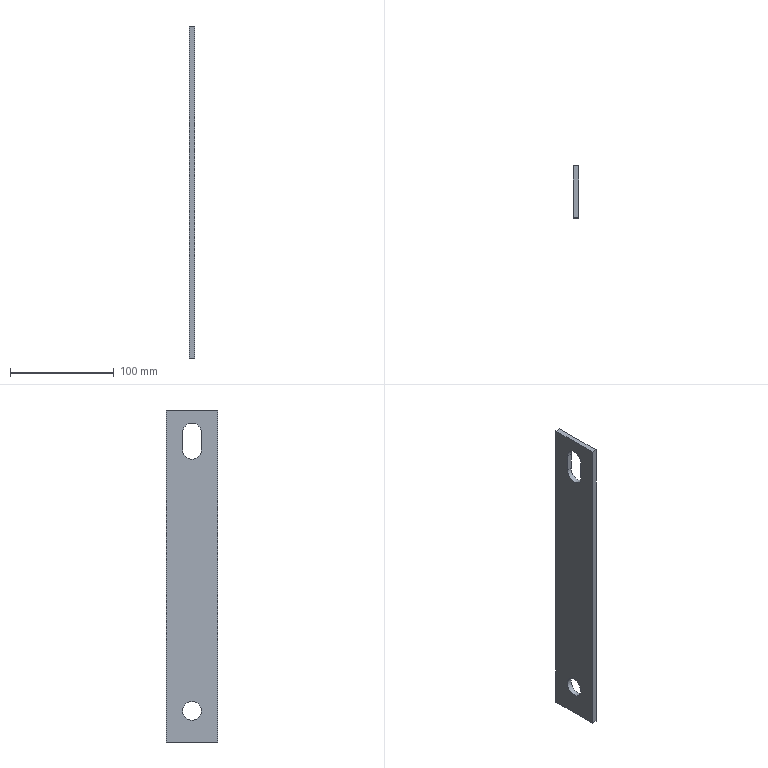Part | NX | features solid 2 | 1 solid | 11 faces | box 5 x 50 x 320 mm | volume 75925 mm3 | plane 8 | cylinder 3 | commonest cylinder face diameters 18 x3
STEP:
#1=CARTESIAN_POINT('',(-1310.,-435.,-90.));
#2=VERTEX_POINT('',#1);
#3=CARTESIAN_POINT('',(-1310.,-485.,-90.));
#4=VERTEX_POINT('',#3);
#5=CARTESIAN_POINT('',(-1310.,-460.,-90.));
#6=DIRECTION('',(0.,-1.,0.));
#7=VECTOR('',#6,1000.);
#8=LINE('',#5,#7);
#9=EDGE_CURVE('',#2,#4,#8,.T.);
#10=ORIENTED_EDGE('',*,*,#9,.T.);
#11=CARTESIAN_POINT('',(-1315.,-485.,-90.));
#12=VERTEX_POINT('',#11);
#13=CARTESIAN_POINT('',(-1312.5,-485.,-90.));
#14=DIRECTION('',(-1.,0.,0.));
#15=VECTOR('',#14,1000.);
#16=LINE('',#13,#15);
#17=EDGE_CURVE('',#4,#12,#16,.T.);
#18=ORIENTED_EDGE('',*,*,#17,.T.);
#19=CARTESIAN_POINT('',(-1315.,-435.,-90.));
#20=VERTEX_POINT('',#19);
#21=CARTESIAN_POINT('',(-1315.,-460.,-90.));
#22=DIRECTION('',(0.,1.,0.));
#23=VECTOR('',#22,1000.);
#24=LINE('',#21,#23);
#25=EDGE_CURVE('',#12,#20,#24,.T.);
#26=ORIENTED_EDGE('',*,*,#25,.T.);
#27=CARTESIAN_POINT('',(-1312.5,-435.,-90.));
#28=DIRECTION('',(1.,0.,0.));
#29=VECTOR('',#28,1000.);
#30=LINE('',#27,#29);
#31=EDGE_CURVE('',#20,#2,#30,.T.);
#32=ORIENTED_EDGE('',*,*,#31,.T.);
#33=EDGE_LOOP('',(#10,#18,#26,#32));
#34=FACE_BOUND('',#33,.T.);
#35=CARTESIAN_POINT('',(-1312.5,-460.,-90.));
#36=DIRECTION('',(0.,0.,-1.));
#37=DIRECTION('',(-1.,0.,0.));
#38=AXIS2_PLACEMENT_3D('',#35,#36,#37);
#39=PLANE('',#38);
#40=ADVANCED_FACE('',(#34),#39,.T.);
#41=CARTESIAN_POINT('',(-1315.,-460.,-69.));
#42=VERTEX_POINT('',#41);
#43=CARTESIAN_POINT('',(-1315.,-460.,-60.));
#44=DIRECTION('',(-1.,0.,0.));
#45=DIRECTION('',(0.,0.,-1.));
#46=AXIS2_PLACEMENT_3D('',#43,#44,#45);
#47=CIRCLE('',#46,9.);
#48=EDGE_CURVE('',#42,#42,#47,.T.);
#49=ORIENTED_EDGE('',*,*,#48,.T.);
#50=EDGE_LOOP('',(#49));
#51=FACE_BOUND('',#50,.T.);
#52=CARTESIAN_POINT('',(-1310.,-460.,-51.));
#53=VERTEX_POINT('',#52);
#54=CARTESIAN_POINT('',(-1310.,-460.,-60.));
#55=DIRECTION('',(1.,0.,0.));
#56=DIRECTION('',(0.,0.,1.));
#57=AXIS2_PLACEMENT_3D('',#54,#55,#56);
#58=CIRCLE('',#57,9.);
#59=EDGE_CURVE('',#53,#53,#58,.T.);
#60=ORIENTED_EDGE('',*,*,#59,.T.);
#61=EDGE_LOOP('',(#60));
#62=FACE_BOUND('',#61,.T.);
#63=CARTESIAN_POINT('',(-1310.,-460.,-60.));
#64=DIRECTION('',(-1.,0.,0.));
#65=DIRECTION('',(0.,0.,1.));
#66=AXIS2_PLACEMENT_3D('',#63,#64,#65);
#67=CYLINDRICAL_SURFACE('',#66,9.);
#68=ADVANCED_FACE('',(#51,#62),#67,.F.);
#69=ORIENTED_EDGE('',*,*,#59,.F.);
#70=EDGE_LOOP('',(#69));
#71=FACE_BOUND('',#70,.T.);
#72=CARTESIAN_POINT('',(-1310.,-485.,230.));
#73=VERTEX_POINT('',#72);
#74=CARTESIAN_POINT('',(-1310.,-485.,-120.));
#75=DIRECTION('',(0.,0.,1.));
#76=VECTOR('',#75,1000.);
#77=LINE('',#74,#76);
#78=EDGE_CURVE('',#4,#73,#77,.T.);
#79=ORIENTED_EDGE('',*,*,#78,.F.);
#80=ORIENTED_EDGE('',*,*,#9,.F.);
#81=CARTESIAN_POINT('',(-1310.,-435.,230.));
#82=VERTEX_POINT('',#81);
#83=CARTESIAN_POINT('',(-1310.,-435.,-120.));
#84=DIRECTION('',(0.,0.,1.));
#85=VECTOR('',#84,1000.);
#86=LINE('',#83,#85);
#87=EDGE_CURVE('',#2,#82,#86,.T.);
#88=ORIENTED_EDGE('',*,*,#87,.T.);
#89=CARTESIAN_POINT('',(-1310.,-460.,230.));
#90=DIRECTION('',(0.,1.,0.));
#91=VECTOR('',#90,1000.);
#92=LINE('',#89,#91);
#93=EDGE_CURVE('',#73,#82,#92,.T.);
#94=ORIENTED_EDGE('',*,*,#93,.F.);
#95=EDGE_LOOP('',(#79,#80,#88,#94));
#96=FACE_BOUND('',#95,.T.);
#97=CARTESIAN_POINT('',(-1310.,-451.,191.5));
#98=VERTEX_POINT('',#97);
#99=CARTESIAN_POINT('',(-1310.,-451.,208.5));
#100=VERTEX_POINT('',#99);
#101=CARTESIAN_POINT('',(-1310.,-451.,191.5));
#102=DIRECTION('',(0.,0.,1.));
#103=VECTOR('',#102,1000.);
#104=LINE('',#101,#103);
#105=EDGE_CURVE('',#98,#100,#104,.T.);
#106=ORIENTED_EDGE('',*,*,#105,.F.);
#107=CARTESIAN_POINT('',(-1310.,-469.,191.5));
#108=VERTEX_POINT('',#107);
#109=CARTESIAN_POINT('',(-1310.,-460.,191.5));
#110=DIRECTION('',(1.,0.,0.));
#111=DIRECTION('',(0.,0.,1.));
#112=AXIS2_PLACEMENT_3D('',#109,#110,#111);
#113=CIRCLE('',#112,9.);
#114=EDGE_CURVE('',#108,#98,#113,.T.);
#115=ORIENTED_EDGE('',*,*,#114,.F.);
#116=CARTESIAN_POINT('',(-1310.,-469.,208.5));
#117=VERTEX_POINT('',#116);
#118=CARTESIAN_POINT('',(-1310.,-469.,191.5));
#119=DIRECTION('',(0.,0.,1.));
#120=VECTOR('',#119,1000.);
#121=LINE('',#118,#120);
#122=EDGE_CURVE('',#108,#117,#121,.T.);
#123=ORIENTED_EDGE('',*,*,#122,.T.);
#124=CARTESIAN_POINT('',(-1310.,-460.,208.5));
#125=DIRECTION('',(1.,0.,0.));
#126=DIRECTION('',(0.,0.,1.));
#127=AXIS2_PLACEMENT_3D('',#124,#125,#126);
#128=CIRCLE('',#127,9.);
#129=EDGE_CURVE('',#100,#117,#128,.T.);
#130=ORIENTED_EDGE('',*,*,#129,.F.);
#131=EDGE_LOOP('',(#106,#115,#123,#130));
#132=FACE_BOUND('',#131,.T.);
#133=CARTESIAN_POINT('',(-1310.,-460.,-120.));
#134=DIRECTION('',(1.,0.,0.));
#135=DIRECTION('',(0.,0.,-1.));
#136=AXIS2_PLACEMENT_3D('',#133,#134,#135);
#137=PLANE('',#136);
#138=ADVANCED_FACE('',(#71,#96,#132),#137,.T.);
#139=CARTESIAN_POINT('',(-1315.,-485.,230.));
#140=VERTEX_POINT('',#139);
#141=CARTESIAN_POINT('',(-1315.,-485.,-120.));
#142=DIRECTION('',(0.,0.,1.));
#143=VECTOR('',#142,1000.);
#144=LINE('',#141,#143);
#145=EDGE_CURVE('',#12,#140,#144,.T.);
#146=ORIENTED_EDGE('',*,*,#145,.F.);
#147=ORIENTED_EDGE('',*,*,#17,.F.);
#148=ORIENTED_EDGE('',*,*,#78,.T.);
#149=CARTESIAN_POINT('',(-1312.5,-485.,230.));
#150=DIRECTION('',(1.,0.,0.));
#151=VECTOR('',#150,1000.);
#152=LINE('',#149,#151);
#153=EDGE_CURVE('',#140,#73,#152,.T.);
#154=ORIENTED_EDGE('',*,*,#153,.F.);
#155=EDGE_LOOP('',(#146,#147,#148,#154));
#156=FACE_BOUND('',#155,.T.);
#157=CARTESIAN_POINT('',(-1312.5,-485.,-120.));
#158=DIRECTION('',(0.,-1.,0.));
#159=DIRECTION('',(0.,0.,1.));
#160=AXIS2_PLACEMENT_3D('',#157,#158,#159);
#161=PLANE('',#160);
#162=ADVANCED_FACE('',(#156),#161,.T.);
#163=ORIENTED_EDGE('',*,*,#48,.F.);
#164=EDGE_LOOP('',(#163));
#165=FACE_BOUND('',#164,.T.);
#166=CARTESIAN_POINT('',(-1315.,-435.,230.));
#167=VERTEX_POINT('',#166);
#168=CARTESIAN_POINT('',(-1315.,-435.,-120.));
#169=DIRECTION('',(0.,0.,1.));
#170=VECTOR('',#169,1000.);
#171=LINE('',#168,#170);
#172=EDGE_CURVE('',#20,#167,#171,.T.);
#173=ORIENTED_EDGE('',*,*,#172,.F.);
#174=ORIENTED_EDGE('',*,*,#25,.F.);
#175=ORIENTED_EDGE('',*,*,#145,.T.);
#176=CARTESIAN_POINT('',(-1315.,-460.,230.));
#177=DIRECTION('',(0.,-1.,0.));
#178=VECTOR('',#177,1000.);
#179=LINE('',#176,#178);
#180=EDGE_CURVE('',#167,#140,#179,.T.);
#181=ORIENTED_EDGE('',*,*,#180,.F.);
#182=EDGE_LOOP('',(#173,#174,#175,#181));
#183=FACE_BOUND('',#182,.T.);
#184=CARTESIAN_POINT('',(-1315.,-451.,191.5));
#185=VERTEX_POINT('',#184);
#186=CARTESIAN_POINT('',(-1315.,-451.,208.5));
#187=VERTEX_POINT('',#186);
#188=CARTESIAN_POINT('',(-1315.,-451.,191.5));
#189=DIRECTION('',(0.,0.,1.));
#190=VECTOR('',#189,1000.);
#191=LINE('',#188,#190);
#192=EDGE_CURVE('',#185,#187,#191,.T.);
#193=ORIENTED_EDGE('',*,*,#192,.T.);
#194=CARTESIAN_POINT('',(-1315.,-469.,208.5));
#195=VERTEX_POINT('',#194);
#196=CARTESIAN_POINT('',(-1315.,-460.,208.5));
#197=DIRECTION('',(-1.,0.,0.));
#198=DIRECTION('',(0.,0.,-1.));
#199=AXIS2_PLACEMENT_3D('',#196,#197,#198);
#200=CIRCLE('',#199,9.);
#201=EDGE_CURVE('',#195,#187,#200,.T.);
#202=ORIENTED_EDGE('',*,*,#201,.F.);
#203=CARTESIAN_POINT('',(-1315.,-469.,191.5));
#204=VERTEX_POINT('',#203);
#205=CARTESIAN_POINT('',(-1315.,-469.,191.5));
#206=DIRECTION('',(0.,0.,1.));
#207=VECTOR('',#206,1000.);
#208=LINE('',#205,#207);
#209=EDGE_CURVE('',#204,#195,#208,.T.);
#210=ORIENTED_EDGE('',*,*,#209,.F.);
#211=CARTESIAN_POINT('',(-1315.,-460.,191.5));
#212=DIRECTION('',(-1.,0.,0.));
#213=DIRECTION('',(0.,0.,-1.));
#214=AXIS2_PLACEMENT_3D('',#211,#212,#213);
#215=CIRCLE('',#214,9.);
#216=EDGE_CURVE('',#185,#204,#215,.T.);
#217=ORIENTED_EDGE('',*,*,#216,.F.);
#218=EDGE_LOOP('',(#193,#202,#210,#217));
#219=FACE_BOUND('',#218,.T.);
#220=CARTESIAN_POINT('',(-1315.,-460.,-120.));
#221=DIRECTION('',(-1.,0.,0.));
#222=DIRECTION('',(0.,0.,1.));
#223=AXIS2_PLACEMENT_3D('',#220,#221,#222);
#224=PLANE('',#223);
#225=ADVANCED_FACE('',(#165,#183,#219),#224,.T.);
#226=ORIENTED_EDGE('',*,*,#87,.F.);
#227=ORIENTED_EDGE('',*,*,#31,.F.);
#228=ORIENTED_EDGE('',*,*,#172,.T.);
#229=CARTESIAN_POINT('',(-1312.5,-435.,230.));
#230=DIRECTION('',(-1.,0.,0.));
#231=VECTOR('',#230,1000.);
#232=LINE('',#229,#231);
#233=EDGE_CURVE('',#82,#167,#232,.T.);
#234=ORIENTED_EDGE('',*,*,#233,.F.);
#235=EDGE_LOOP('',(#226,#227,#228,#234));
#236=FACE_BOUND('',#235,.T.);
#237=CARTESIAN_POINT('',(-1312.5,-435.,-120.));
#238=DIRECTION('',(0.,1.,0.));
#239=DIRECTION('',(0.,0.,-1.));
#240=AXIS2_PLACEMENT_3D('',#237,#238,#239);
#241=PLANE('',#240);
#242=ADVANCED_FACE('',(#236),#241,.T.);
#243=CARTESIAN_POINT('',(-1312.5,-451.,208.5));
#244=DIRECTION('',(-1.,0.,0.));
#245=VECTOR('',#244,1000.);
#246=LINE('',#243,#245);
#247=EDGE_CURVE('',#100,#187,#246,.T.);
#248=ORIENTED_EDGE('',*,*,#247,.F.);
#249=ORIENTED_EDGE('',*,*,#129,.T.);
#250=CARTESIAN_POINT('',(-1312.5,-469.,208.5));
#251=DIRECTION('',(1.,0.,0.));
#252=VECTOR('',#251,1000.);
#253=LINE('',#250,#252);
#254=EDGE_CURVE('',#195,#117,#253,.T.);
#255=ORIENTED_EDGE('',*,*,#254,.F.);
#256=ORIENTED_EDGE('',*,*,#201,.T.);
#257=EDGE_LOOP('',(#248,#249,#255,#256));
#258=FACE_BOUND('',#257,.T.);
#259=CARTESIAN_POINT('',(-1310.,-460.,208.5));
#260=DIRECTION('',(-1.,0.,0.));
#261=DIRECTION('',(0.,0.,1.));
#262=AXIS2_PLACEMENT_3D('',#259,#260,#261);
#263=CYLINDRICAL_SURFACE('',#262,9.);
#264=ADVANCED_FACE('',(#258),#263,.F.);
#265=ORIENTED_EDGE('',*,*,#233,.T.);
#266=ORIENTED_EDGE('',*,*,#180,.T.);
#267=ORIENTED_EDGE('',*,*,#153,.T.);
#268=ORIENTED_EDGE('',*,*,#93,.T.);
#269=EDGE_LOOP('',(#265,#266,#267,#268));
#270=FACE_BOUND('',#269,.T.);
#271=CARTESIAN_POINT('',(-1302.5,-460.,230.));
#272=DIRECTION('',(0.,0.,1.));
#273=DIRECTION('',(1.,0.,0.));
#274=AXIS2_PLACEMENT_3D('',#271,#272,#273);
#275=PLANE('',#274);
#276=ADVANCED_FACE('',(#270),#275,.T.);
#277=ORIENTED_EDGE('',*,*,#216,.T.);
#278=CARTESIAN_POINT('',(-1312.5,-469.,191.5));
#279=DIRECTION('',(-1.,0.,0.));
#280=VECTOR('',#279,1000.);
#281=LINE('',#278,#280);
#282=EDGE_CURVE('',#108,#204,#281,.T.);
#283=ORIENTED_EDGE('',*,*,#282,.F.);
#284=ORIENTED_EDGE('',*,*,#114,.T.);
#285=CARTESIAN_POINT('',(-1312.5,-451.,191.5));
#286=DIRECTION('',(1.,0.,0.));
#287=VECTOR('',#286,1000.);
#288=LINE('',#285,#287);
#289=EDGE_CURVE('',#185,#98,#288,.T.);
#290=ORIENTED_EDGE('',*,*,#289,.F.);
#291=EDGE_LOOP('',(#277,#283,#284,#290));
#292=FACE_BOUND('',#291,.T.);
#293=CARTESIAN_POINT('',(-1310.,-460.,191.5));
#294=DIRECTION('',(-1.,0.,0.));
#295=DIRECTION('',(0.,0.,1.));
#296=AXIS2_PLACEMENT_3D('',#293,#294,#295);
#297=CYLINDRICAL_SURFACE('',#296,9.);
#298=ADVANCED_FACE('',(#292),#297,.F.);
#299=ORIENTED_EDGE('',*,*,#209,.T.);
#300=ORIENTED_EDGE('',*,*,#254,.T.);
#301=ORIENTED_EDGE('',*,*,#122,.F.);
#302=ORIENTED_EDGE('',*,*,#282,.T.);
#303=EDGE_LOOP('',(#299,#300,#301,#302));
#304=FACE_BOUND('',#303,.T.);
#305=CARTESIAN_POINT('',(-1312.5,-469.,191.5));
#306=DIRECTION('',(0.,-1.,0.));
#307=DIRECTION('',(0.,0.,1.));
#308=AXIS2_PLACEMENT_3D('',#305,#306,#307);
#309=PLANE('',#308);
#310=ADVANCED_FACE('',(#304),#309,.F.);
#311=ORIENTED_EDGE('',*,*,#105,.T.);
#312=ORIENTED_EDGE('',*,*,#247,.T.);
#313=ORIENTED_EDGE('',*,*,#192,.F.);
#314=ORIENTED_EDGE('',*,*,#289,.T.);
#315=EDGE_LOOP('',(#311,#312,#313,#314));
#316=FACE_BOUND('',#315,.T.);
#317=CARTESIAN_POINT('',(-1312.5,-451.,191.5));
#318=DIRECTION('',(0.,1.,0.));
#319=DIRECTION('',(0.,0.,-1.));
#320=AXIS2_PLACEMENT_3D('',#317,#318,#319);
#321=PLANE('',#320);
#322=ADVANCED_FACE('',(#316),#321,.F.);
#323=CLOSED_SHELL('',(#40,#68,#138,#162,#225,#242,#264,#276,#298,#310,#322));
#324=MANIFOLD_SOLID_BREP('',#323);
#325=(LENGTH_UNIT()NAMED_UNIT(*)SI_UNIT(.MILLI.,.METRE.));
#326=UNCERTAINTY_MEASURE_WITH_UNIT(LENGTH_MEASURE(0.00001),#325,'','');
#327=(NAMED_UNIT(*)PLANE_ANGLE_UNIT()SI_UNIT($,.RADIAN.));
#328=(NAMED_UNIT(*)SI_UNIT($,.STERADIAN.)SOLID_ANGLE_UNIT());
#329=(GEOMETRIC_REPRESENTATION_CONTEXT(3)GLOBAL_UNCERTAINTY_ASSIGNED_CONTEXT((#326))GLOBAL_UNIT_ASSIGNED_CONTEXT((#325,#327,#328))REPRESENTATION_CONTEXT('',''));
#330=ADVANCED_BREP_SHAPE_REPRESENTATION('',(#324),#329);